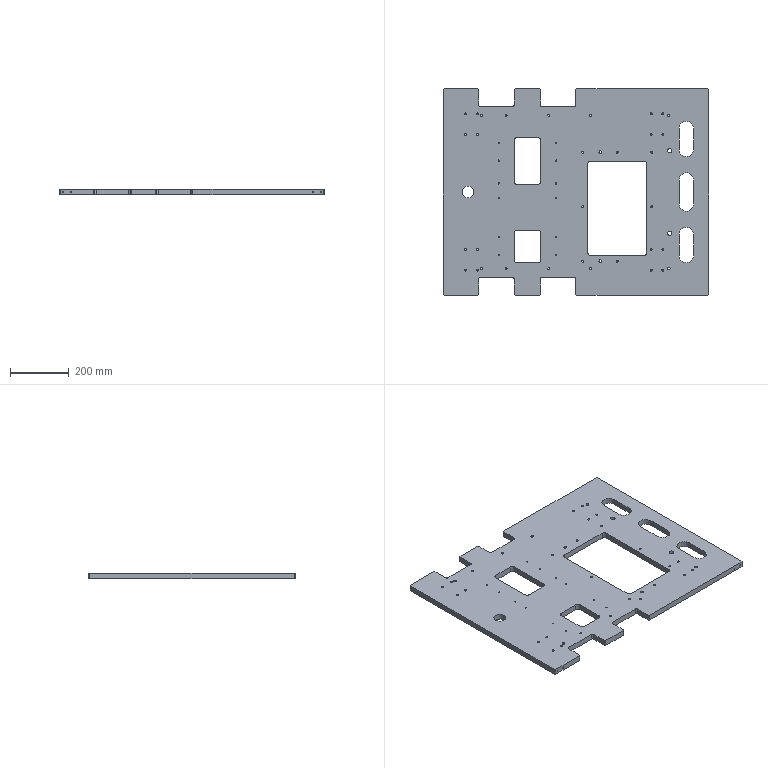Part | STEP file | PN_0022 Base Default | 1 solid | 418 faces | box 900 x 700 x 20 mm | volume 9845455 mm3 | cylinder 244 | cone 116 | plane 58 | commonest cylinder face diameters 4.2 x70 6.8 x54 3.3 x28 5 x28 9 x16 10 x12